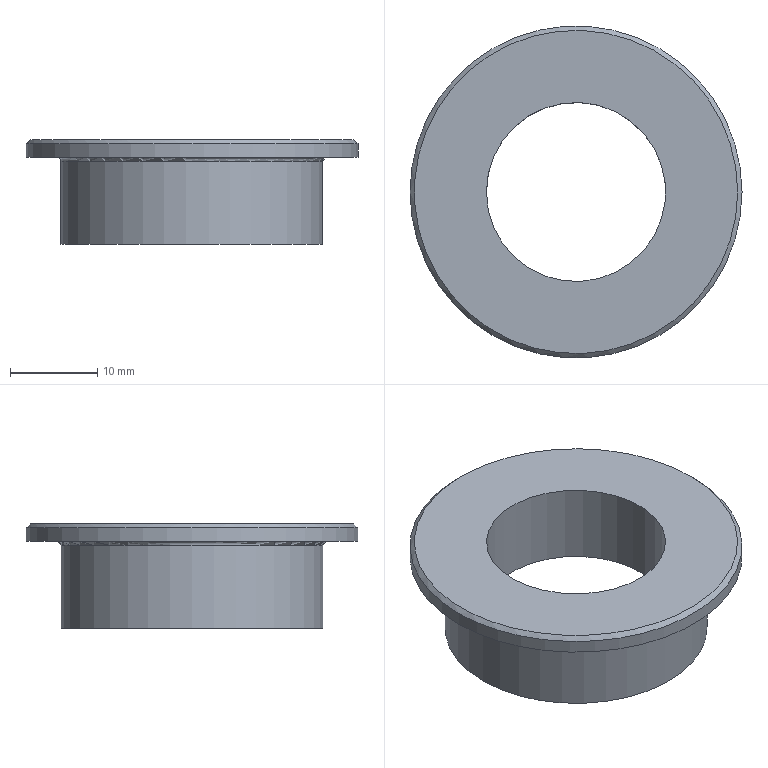Part | NX | features DATUM_CSYS 2, BLEND 1, CHAMFER 1, SKETCH 1, SWP104 1 | 1 solid | 8 faces | box 38 x 38 x 12 mm | volume 4882 mm3 | cylinder 3 | cone 2 | plane 2 | torus 1 | commonest cylinder face diameters 20.5 x1 30 x1 38 x1
STEP:
#1=CARTESIAN_POINT('',(-10.25,0.,2.742));
#2=VERTEX_POINT('',#1);
#3=CARTESIAN_POINT('',(0.,0.,2.742));
#4=DIRECTION('',(0.,0.,-1.));
#5=DIRECTION('',(-1.,0.,0.));
#6=AXIS2_PLACEMENT_3D('',#3,#4,#5);
#7=CIRCLE('',#6,10.25);
#8=EDGE_CURVE('',#2,#2,#7,.T.);
#9=ORIENTED_EDGE('',*,*,#8,.T.);
#10=EDGE_LOOP('',(#9));
#11=FACE_BOUND('',#10,.T.);
#12=CARTESIAN_POINT('',(-10.25,0.,12.));
#13=VERTEX_POINT('',#12);
#14=CARTESIAN_POINT('',(0.,0.,12.));
#15=DIRECTION('',(0.,0.,-1.));
#16=DIRECTION('',(-1.,0.,0.));
#17=AXIS2_PLACEMENT_3D('',#14,#15,#16);
#18=CIRCLE('',#17,10.25);
#19=EDGE_CURVE('',#13,#13,#18,.T.);
#20=ORIENTED_EDGE('',*,*,#19,.F.);
#21=EDGE_LOOP('',(#20));
#22=FACE_BOUND('',#21,.T.);
#23=CARTESIAN_POINT('',(0.,0.,0.));
#24=DIRECTION('',(0.,0.,-1.));
#25=DIRECTION('',(-1.,0.,0.));
#26=AXIS2_PLACEMENT_3D('',#23,#24,#25);
#27=CYLINDRICAL_SURFACE('',#26,10.25);
#28=ADVANCED_FACE('',(#11,#22),#27,.F.);
#29=CARTESIAN_POINT('',(-15.,0.,0.));
#30=VERTEX_POINT('',#29);
#31=CARTESIAN_POINT('',(0.,0.,0.));
#32=DIRECTION('',(0.,0.,-1.));
#33=DIRECTION('',(-1.,0.,0.));
#34=AXIS2_PLACEMENT_3D('',#31,#32,#33);
#35=CIRCLE('',#34,15.);
#36=EDGE_CURVE('',#30,#30,#35,.T.);
#37=ORIENTED_EDGE('',*,*,#36,.T.);
#38=EDGE_LOOP('',(#37));
#39=FACE_BOUND('',#38,.T.);
#40=ORIENTED_EDGE('',*,*,#8,.F.);
#41=EDGE_LOOP('',(#40));
#42=FACE_BOUND('',#41,.T.);
#43=CARTESIAN_POINT('',(0.,0.,2.742));
#44=DIRECTION('',(0.,0.,-1.));
#45=DIRECTION('',(-1.,0.,0.));
#46=AXIS2_PLACEMENT_3D('',#43,#44,#45);
#47=CONICAL_SURFACE('',#46,10.25,1.047);
#48=ADVANCED_FACE('',(#39,#42),#47,.F.);
#49=CARTESIAN_POINT('',(-15.,0.,9.5));
#50=VERTEX_POINT('',#49);
#51=CARTESIAN_POINT('',(0.,0.,9.5));
#52=DIRECTION('',(0.,0.,-1.));
#53=DIRECTION('',(-1.,0.,0.));
#54=AXIS2_PLACEMENT_3D('',#51,#52,#53);
#55=CIRCLE('',#54,15.);
#56=EDGE_CURVE('',#50,#50,#55,.T.);
#57=ORIENTED_EDGE('',*,*,#56,.T.);
#58=EDGE_LOOP('',(#57));
#59=FACE_BOUND('',#58,.T.);
#60=ORIENTED_EDGE('',*,*,#36,.F.);
#61=EDGE_LOOP('',(#60));
#62=FACE_BOUND('',#61,.T.);
#63=CARTESIAN_POINT('',(0.,0.,0.));
#64=DIRECTION('',(0.,0.,-1.));
#65=DIRECTION('',(-1.,0.,0.));
#66=AXIS2_PLACEMENT_3D('',#63,#64,#65);
#67=CYLINDRICAL_SURFACE('',#66,15.);
#68=ADVANCED_FACE('',(#59,#62),#67,.T.);
#69=CARTESIAN_POINT('',(-15.5,0.,10.));
#70=VERTEX_POINT('',#69);
#71=CARTESIAN_POINT('',(0.,0.,10.));
#72=DIRECTION('',(0.,0.,-1.));
#73=DIRECTION('',(-1.,0.,0.));
#74=AXIS2_PLACEMENT_3D('',#71,#72,#73);
#75=CIRCLE('',#74,15.5);
#76=EDGE_CURVE('',#70,#70,#75,.F.);
#77=ORIENTED_EDGE('',*,*,#76,.T.);
#78=EDGE_LOOP('',(#77));
#79=FACE_BOUND('',#78,.T.);
#80=CARTESIAN_POINT('',(-19.,0.,10.));
#81=VERTEX_POINT('',#80);
#82=CARTESIAN_POINT('',(0.,0.,10.));
#83=DIRECTION('',(0.,0.,-1.));
#84=DIRECTION('',(-1.,0.,0.));
#85=AXIS2_PLACEMENT_3D('',#82,#83,#84);
#86=CIRCLE('',#85,19.);
#87=EDGE_CURVE('',#81,#81,#86,.T.);
#88=ORIENTED_EDGE('',*,*,#87,.T.);
#89=EDGE_LOOP('',(#88));
#90=FACE_BOUND('',#89,.T.);
#91=CARTESIAN_POINT('',(15.,0.,10.));
#92=DIRECTION('',(0.,0.,-1.));
#93=DIRECTION('',(-1.,0.,0.));
#94=AXIS2_PLACEMENT_3D('',#91,#92,#93);
#95=PLANE('',#94);
#96=ADVANCED_FACE('',(#79,#90),#95,.T.);
#97=CARTESIAN_POINT('',(19.,0.,11.5));
#98=VERTEX_POINT('',#97);
#99=CARTESIAN_POINT('',(0.,0.,11.5));
#100=DIRECTION('',(0.,0.,1.));
#101=DIRECTION('',(1.,0.,0.));
#102=AXIS2_PLACEMENT_3D('',#99,#100,#101);
#103=CIRCLE('',#102,19.);
#104=EDGE_CURVE('',#98,#98,#103,.F.);
#105=ORIENTED_EDGE('',*,*,#104,.T.);
#106=EDGE_LOOP('',(#105));
#107=FACE_BOUND('',#106,.T.);
#108=ORIENTED_EDGE('',*,*,#87,.F.);
#109=EDGE_LOOP('',(#108));
#110=FACE_BOUND('',#109,.T.);
#111=CARTESIAN_POINT('',(0.,0.,0.));
#112=DIRECTION('',(0.,0.,-1.));
#113=DIRECTION('',(-1.,0.,0.));
#114=AXIS2_PLACEMENT_3D('',#111,#112,#113);
#115=CYLINDRICAL_SURFACE('',#114,19.);
#116=ADVANCED_FACE('',(#107,#110),#115,.T.);
#117=CARTESIAN_POINT('',(18.5,0.,12.));
#118=VERTEX_POINT('',#117);
#119=CARTESIAN_POINT('',(0.,0.,12.));
#120=DIRECTION('',(0.,0.,1.));
#121=DIRECTION('',(1.,0.,0.));
#122=AXIS2_PLACEMENT_3D('',#119,#120,#121);
#123=CIRCLE('',#122,18.5);
#124=EDGE_CURVE('',#118,#118,#123,.T.);
#125=ORIENTED_EDGE('',*,*,#124,.T.);
#126=EDGE_LOOP('',(#125));
#127=FACE_BOUND('',#126,.T.);
#128=ORIENTED_EDGE('',*,*,#19,.T.);
#129=EDGE_LOOP('',(#128));
#130=FACE_BOUND('',#129,.T.);
#131=CARTESIAN_POINT('',(19.,0.,12.));
#132=DIRECTION('',(0.,0.,1.));
#133=DIRECTION('',(1.,0.,0.));
#134=AXIS2_PLACEMENT_3D('',#131,#132,#133);
#135=PLANE('',#134);
#136=ADVANCED_FACE('',(#127,#130),#135,.T.);
#137=ORIENTED_EDGE('',*,*,#76,.F.);
#138=EDGE_LOOP('',(#137));
#139=FACE_BOUND('',#138,.T.);
#140=ORIENTED_EDGE('',*,*,#56,.F.);
#141=EDGE_LOOP('',(#140));
#142=FACE_BOUND('',#141,.T.);
#143=CARTESIAN_POINT('',(0.,0.,9.5));
#144=DIRECTION('',(0.,0.,-1.));
#145=DIRECTION('',(-1.,0.,0.));
#146=AXIS2_PLACEMENT_3D('',#143,#144,#145);
#147=TOROIDAL_SURFACE('',#146,15.5,0.5);
#148=ADVANCED_FACE('',(#139,#142),#147,.F.);
#149=ORIENTED_EDGE('',*,*,#124,.F.);
#150=EDGE_LOOP('',(#149));
#151=FACE_BOUND('',#150,.T.);
#152=ORIENTED_EDGE('',*,*,#104,.F.);
#153=EDGE_LOOP('',(#152));
#154=FACE_BOUND('',#153,.T.);
#155=CARTESIAN_POINT('',(0.,0.,11.5));
#156=DIRECTION('',(0.,0.,-1.));
#157=DIRECTION('',(-1.,0.,0.));
#158=AXIS2_PLACEMENT_3D('',#155,#156,#157);
#159=CONICAL_SURFACE('',#158,19.,0.7854);
#160=ADVANCED_FACE('',(#151,#154),#159,.T.);
#161=CLOSED_SHELL('',(#28,#48,#68,#96,#116,#136,#148,#160));
#162=MANIFOLD_SOLID_BREP('',#161);
#163=(LENGTH_UNIT()NAMED_UNIT(*)SI_UNIT(.MILLI.,.METRE.));
#164=UNCERTAINTY_MEASURE_WITH_UNIT(LENGTH_MEASURE(0.00001),#163,'','');
#165=(NAMED_UNIT(*)PLANE_ANGLE_UNIT()SI_UNIT($,.RADIAN.));
#166=(NAMED_UNIT(*)SI_UNIT($,.STERADIAN.)SOLID_ANGLE_UNIT());
#167=(GEOMETRIC_REPRESENTATION_CONTEXT(3)GLOBAL_UNCERTAINTY_ASSIGNED_CONTEXT((#164))GLOBAL_UNIT_ASSIGNED_CONTEXT((#163,#165,#166))REPRESENTATION_CONTEXT('',''));
#168=ADVANCED_BREP_SHAPE_REPRESENTATION('',(#162),#167);